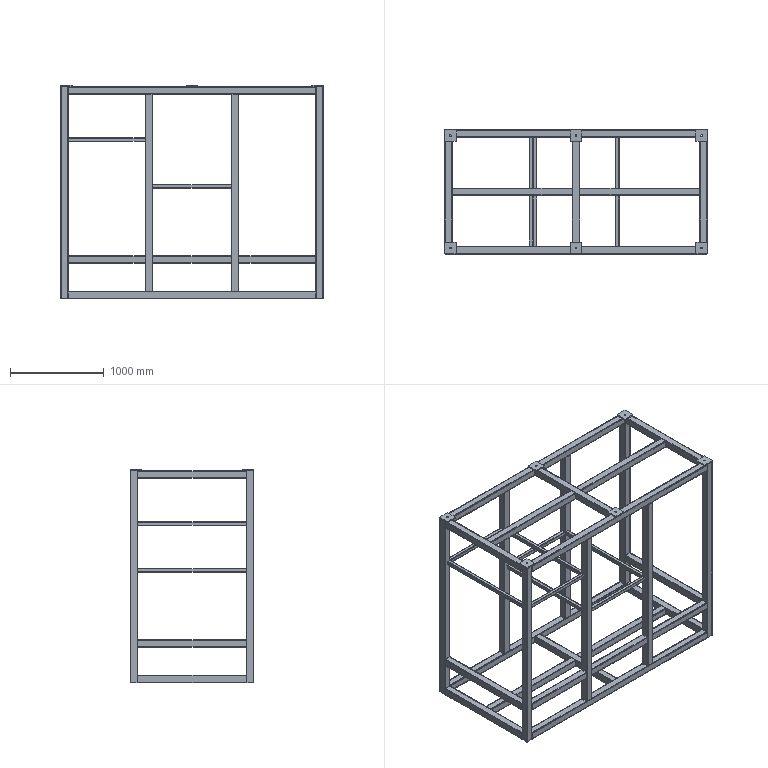Part | STEP file | Part5_default<as machined> | 41 solids | 682 faces | box 2800 x 1320 x 2280 mm | volume 46678246 mm3 | plane 386 | cylinder 296 | commonest cylinder face diameters 6.4 x108 12.8 x108 4 x32 8 x32 17.5 x16